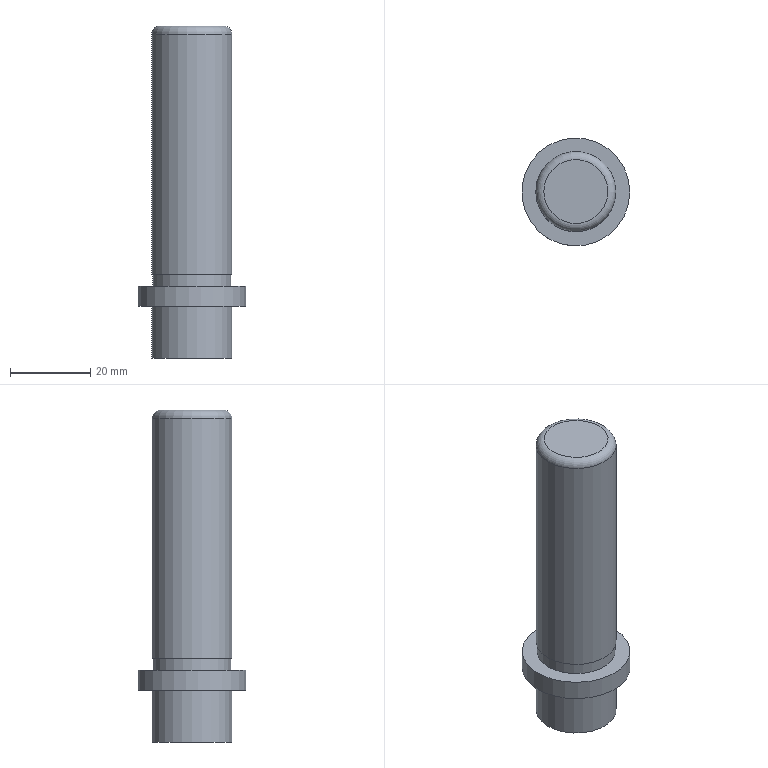Part | NX | features 1 2 | 1 solid | 14 faces | box 27 x 27 x 83 mm | volume 26117 mm3 | cylinder 6 | plane 5 | cone 2 | torus 1 | commonest cylinder face diameters 20 x2 6.8 x1 8 x1 19.5 x1 27 x1
STEP:
#1=CARTESIAN_POINT('',(336.,108.,27.));
#2=VERTEX_POINT('',#1);
#3=CARTESIAN_POINT('',(326.,108.,27.));
#4=DIRECTION('',(0.,0.,1.));
#5=DIRECTION('',(1.,0.,0.));
#6=AXIS2_PLACEMENT_3D('',#3,#4,#5);
#7=CIRCLE('',#6,10.);
#8=EDGE_CURVE('',#2,#2,#7,.T.);
#9=ORIENTED_EDGE('',*,*,#8,.T.);
#10=EDGE_LOOP('',(#9));
#11=FACE_BOUND('',#10,.T.);
#12=CARTESIAN_POINT('',(336.,108.,40.));
#13=VERTEX_POINT('',#12);
#14=CARTESIAN_POINT('',(326.,108.,40.));
#15=DIRECTION('',(0.,0.,1.));
#16=DIRECTION('',(1.,0.,0.));
#17=AXIS2_PLACEMENT_3D('',#14,#15,#16);
#18=CIRCLE('',#17,10.);
#19=EDGE_CURVE('',#13,#13,#18,.T.);
#20=ORIENTED_EDGE('',*,*,#19,.F.);
#21=EDGE_LOOP('',(#20));
#22=FACE_BOUND('',#21,.T.);
#23=CARTESIAN_POINT('',(326.,108.,67.));
#24=DIRECTION('',(0.,0.,1.));
#25=DIRECTION('',(-1.,0.,0.));
#26=AXIS2_PLACEMENT_3D('',#23,#24,#25);
#27=CYLINDRICAL_SURFACE('',#26,10.);
#28=ADVANCED_FACE('',(#11,#22),#27,.T.);
#29=CARTESIAN_POINT('',(339.5,108.,40.));
#30=VERTEX_POINT('',#29);
#31=CARTESIAN_POINT('',(326.,108.,40.));
#32=DIRECTION('',(0.,0.,1.));
#33=DIRECTION('',(1.,0.,0.));
#34=AXIS2_PLACEMENT_3D('',#31,#32,#33);
#35=CIRCLE('',#34,13.5);
#36=EDGE_CURVE('',#30,#30,#35,.T.);
#37=ORIENTED_EDGE('',*,*,#36,.T.);
#38=EDGE_LOOP('',(#37));
#39=FACE_BOUND('',#38,.T.);
#40=CARTESIAN_POINT('',(339.5,108.,45.));
#41=VERTEX_POINT('',#40);
#42=CARTESIAN_POINT('',(326.,108.,45.));
#43=DIRECTION('',(0.,0.,-1.));
#44=DIRECTION('',(1.,0.,0.));
#45=AXIS2_PLACEMENT_3D('',#42,#43,#44);
#46=CIRCLE('',#45,13.5);
#47=EDGE_CURVE('',#41,#41,#46,.T.);
#48=ORIENTED_EDGE('',*,*,#47,.T.);
#49=EDGE_LOOP('',(#48));
#50=FACE_BOUND('',#49,.T.);
#51=CARTESIAN_POINT('',(326.,108.,42.5));
#52=DIRECTION('',(0.,0.,1.));
#53=DIRECTION('',(-1.,0.,0.));
#54=AXIS2_PLACEMENT_3D('',#51,#52,#53);
#55=CYLINDRICAL_SURFACE('',#54,13.5);
#56=ADVANCED_FACE('',(#39,#50),#55,.T.);
#57=CARTESIAN_POINT('',(335.75,108.,45.));
#58=VERTEX_POINT('',#57);
#59=CARTESIAN_POINT('',(326.,108.,45.));
#60=DIRECTION('',(0.,0.,-1.));
#61=DIRECTION('',(1.,0.,0.));
#62=AXIS2_PLACEMENT_3D('',#59,#60,#61);
#63=CIRCLE('',#62,9.75);
#64=EDGE_CURVE('',#58,#58,#63,.T.);
#65=ORIENTED_EDGE('',*,*,#64,.F.);
#66=EDGE_LOOP('',(#65));
#67=FACE_BOUND('',#66,.T.);
#68=CARTESIAN_POINT('',(335.75,108.,48.));
#69=VERTEX_POINT('',#68);
#70=CARTESIAN_POINT('',(326.,108.,48.));
#71=DIRECTION('',(0.,0.,1.));
#72=DIRECTION('',(1.,0.,0.));
#73=AXIS2_PLACEMENT_3D('',#70,#71,#72);
#74=CIRCLE('',#73,9.75);
#75=EDGE_CURVE('',#69,#69,#74,.T.);
#76=ORIENTED_EDGE('',*,*,#75,.F.);
#77=EDGE_LOOP('',(#76));
#78=FACE_BOUND('',#77,.T.);
#79=CARTESIAN_POINT('',(326.,108.,46.5));
#80=DIRECTION('',(0.,0.,1.));
#81=DIRECTION('',(-1.,0.,0.));
#82=AXIS2_PLACEMENT_3D('',#79,#80,#81);
#83=CYLINDRICAL_SURFACE('',#82,9.75);
#84=ADVANCED_FACE('',(#67,#78),#83,.T.);
#85=CARTESIAN_POINT('',(330.,108.,47.));
#86=VERTEX_POINT('',#85);
#87=CARTESIAN_POINT('',(326.,108.,47.));
#88=DIRECTION('',(0.,0.,-1.));
#89=DIRECTION('',(1.,0.,0.));
#90=AXIS2_PLACEMENT_3D('',#87,#88,#89);
#91=CIRCLE('',#90,4.);
#92=EDGE_CURVE('',#86,#86,#91,.T.);
#93=ORIENTED_EDGE('',*,*,#92,.F.);
#94=EDGE_LOOP('',(#93));
#95=FACE_BOUND('',#94,.T.);
#96=CARTESIAN_POINT('',(330.,108.,27.));
#97=VERTEX_POINT('',#96);
#98=CARTESIAN_POINT('',(326.,108.,27.));
#99=DIRECTION('',(0.,0.,-1.));
#100=DIRECTION('',(1.,0.,0.));
#101=AXIS2_PLACEMENT_3D('',#98,#99,#100);
#102=CIRCLE('',#101,4.);
#103=EDGE_CURVE('',#97,#97,#102,.T.);
#104=ORIENTED_EDGE('',*,*,#103,.T.);
#105=EDGE_LOOP('',(#104));
#106=FACE_BOUND('',#105,.T.);
#107=CARTESIAN_POINT('',(326.,108.,37.));
#108=DIRECTION('',(0.,0.,1.));
#109=DIRECTION('',(-1.,0.,0.));
#110=AXIS2_PLACEMENT_3D('',#107,#108,#109);
#111=CYLINDRICAL_SURFACE('',#110,4.);
#112=ADVANCED_FACE('',(#95,#106),#111,.F.);
#113=CARTESIAN_POINT('',(329.4,108.,47.5));
#114=VERTEX_POINT('',#113);
#115=CARTESIAN_POINT('',(326.,108.,47.5));
#116=DIRECTION('',(0.,0.,-1.));
#117=DIRECTION('',(1.,0.,0.));
#118=AXIS2_PLACEMENT_3D('',#115,#116,#117);
#119=CIRCLE('',#118,3.4);
#120=EDGE_CURVE('',#114,#114,#119,.T.);
#121=ORIENTED_EDGE('',*,*,#120,.F.);
#122=EDGE_LOOP('',(#121));
#123=FACE_BOUND('',#122,.T.);
#124=ORIENTED_EDGE('',*,*,#92,.T.);
#125=EDGE_LOOP('',(#124));
#126=FACE_BOUND('',#125,.T.);
#127=CARTESIAN_POINT('',(326.,108.,47.25));
#128=DIRECTION('',(0.,0.,-1.));
#129=DIRECTION('',(-1.,0.,0.));
#130=AXIS2_PLACEMENT_3D('',#127,#128,#129);
#131=CONICAL_SURFACE('',#130,3.7,0.8761);
#132=ADVANCED_FACE('',(#123,#126),#131,.F.);
#133=CARTESIAN_POINT('',(329.4,108.,49.));
#134=VERTEX_POINT('',#133);
#135=CARTESIAN_POINT('',(326.,108.,49.));
#136=DIRECTION('',(0.,0.,-1.));
#137=DIRECTION('',(1.,0.,0.));
#138=AXIS2_PLACEMENT_3D('',#135,#136,#137);
#139=CIRCLE('',#138,3.4);
#140=EDGE_CURVE('',#134,#134,#139,.T.);
#141=ORIENTED_EDGE('',*,*,#140,.F.);
#142=EDGE_LOOP('',(#141));
#143=FACE_BOUND('',#142,.T.);
#144=ORIENTED_EDGE('',*,*,#120,.T.);
#145=EDGE_LOOP('',(#144));
#146=FACE_BOUND('',#145,.T.);
#147=CARTESIAN_POINT('',(326.,108.,48.25));
#148=DIRECTION('',(0.,0.,1.));
#149=DIRECTION('',(-1.,0.,0.));
#150=AXIS2_PLACEMENT_3D('',#147,#148,#149);
#151=CYLINDRICAL_SURFACE('',#150,3.4);
#152=ADVANCED_FACE('',(#143,#146),#151,.F.);
#153=ORIENTED_EDGE('',*,*,#140,.T.);
#154=EDGE_LOOP('',(#153));
#155=FACE_BOUND('',#154,.T.);
#156=CARTESIAN_POINT('',(326.,108.,54.889));
#157=VERTEX_POINT('',#156);
#158=VERTEX_LOOP('',#157);
#159=FACE_BOUND('',#158,.T.);
#160=CARTESIAN_POINT('',(326.,108.,51.944));
#161=DIRECTION('',(0.,0.,-1.));
#162=DIRECTION('',(-1.,0.,0.));
#163=AXIS2_PLACEMENT_3D('',#160,#161,#162);
#164=CONICAL_SURFACE('',#163,1.7,0.5236);
#165=ADVANCED_FACE('',(#155,#159),#164,.F.);
#166=CARTESIAN_POINT('',(336.,108.,48.));
#167=VERTEX_POINT('',#166);
#168=CARTESIAN_POINT('',(326.,108.,48.));
#169=DIRECTION('',(0.,0.,-1.));
#170=DIRECTION('',(1.,0.,0.));
#171=AXIS2_PLACEMENT_3D('',#168,#169,#170);
#172=CIRCLE('',#171,10.);
#173=EDGE_CURVE('',#167,#167,#172,.T.);
#174=ORIENTED_EDGE('',*,*,#173,.F.);
#175=EDGE_LOOP('',(#174));
#176=FACE_BOUND('',#175,.T.);
#177=CARTESIAN_POINT('',(316.,108.,108.));
#178=VERTEX_POINT('',#177);
#179=CARTESIAN_POINT('',(326.,108.,108.));
#180=DIRECTION('',(0.,0.,1.));
#181=DIRECTION('',(-1.,0.,0.));
#182=AXIS2_PLACEMENT_3D('',#179,#180,#181);
#183=CIRCLE('',#182,10.);
#184=EDGE_CURVE('',#178,#178,#183,.F.);
#185=ORIENTED_EDGE('',*,*,#184,.T.);
#186=EDGE_LOOP('',(#185));
#187=FACE_BOUND('',#186,.T.);
#188=CARTESIAN_POINT('',(326.,108.,67.));
#189=DIRECTION('',(0.,0.,1.));
#190=DIRECTION('',(-1.,0.,0.));
#191=AXIS2_PLACEMENT_3D('',#188,#189,#190);
#192=CYLINDRICAL_SURFACE('',#191,10.);
#193=ADVANCED_FACE('',(#176,#187),#192,.T.);
#194=ORIENTED_EDGE('',*,*,#184,.F.);
#195=EDGE_LOOP('',(#194));
#196=FACE_BOUND('',#195,.T.);
#197=CARTESIAN_POINT('',(318.,108.,110.));
#198=VERTEX_POINT('',#197);
#199=CARTESIAN_POINT('',(326.,108.,110.));
#200=DIRECTION('',(0.,0.,1.));
#201=DIRECTION('',(-1.,0.,0.));
#202=AXIS2_PLACEMENT_3D('',#199,#200,#201);
#203=CIRCLE('',#202,8.);
#204=EDGE_CURVE('',#198,#198,#203,.T.);
#205=ORIENTED_EDGE('',*,*,#204,.F.);
#206=EDGE_LOOP('',(#205));
#207=FACE_BOUND('',#206,.T.);
#208=CARTESIAN_POINT('',(326.,108.,108.));
#209=DIRECTION('',(0.,0.,-1.));
#210=DIRECTION('',(-1.,0.,0.));
#211=AXIS2_PLACEMENT_3D('',#208,#209,#210);
#212=TOROIDAL_SURFACE('',#211,8.,2.);
#213=ADVANCED_FACE('',(#196,#207),#212,.T.);
#214=ORIENTED_EDGE('',*,*,#204,.T.);
#215=EDGE_LOOP('',(#214));
#216=FACE_BOUND('',#215,.T.);
#217=CARTESIAN_POINT('',(326.,108.,110.));
#218=DIRECTION('',(0.,0.,-1.));
#219=DIRECTION('',(1.,0.,0.));
#220=AXIS2_PLACEMENT_3D('',#217,#218,#219);
#221=PLANE('',#220);
#222=ADVANCED_FACE('',(#216),#221,.F.);
#223=ORIENTED_EDGE('',*,*,#75,.T.);
#224=EDGE_LOOP('',(#223));
#225=FACE_BOUND('',#224,.T.);
#226=ORIENTED_EDGE('',*,*,#173,.T.);
#227=EDGE_LOOP('',(#226));
#228=FACE_BOUND('',#227,.T.);
#229=CARTESIAN_POINT('',(326.,108.,48.));
#230=DIRECTION('',(0.,0.,1.));
#231=DIRECTION('',(-1.,0.,0.));
#232=AXIS2_PLACEMENT_3D('',#229,#230,#231);
#233=PLANE('',#232);
#234=ADVANCED_FACE('',(#225,#228),#233,.F.);
#235=ORIENTED_EDGE('',*,*,#36,.F.);
#236=EDGE_LOOP('',(#235));
#237=FACE_BOUND('',#236,.T.);
#238=ORIENTED_EDGE('',*,*,#19,.T.);
#239=EDGE_LOOP('',(#238));
#240=FACE_BOUND('',#239,.T.);
#241=CARTESIAN_POINT('',(326.,108.,40.));
#242=DIRECTION('',(0.,0.,-1.));
#243=DIRECTION('',(1.,0.,0.));
#244=AXIS2_PLACEMENT_3D('',#241,#242,#243);
#245=PLANE('',#244);
#246=ADVANCED_FACE('',(#237,#240),#245,.T.);
#247=ORIENTED_EDGE('',*,*,#64,.T.);
#248=EDGE_LOOP('',(#247));
#249=FACE_BOUND('',#248,.T.);
#250=ORIENTED_EDGE('',*,*,#47,.F.);
#251=EDGE_LOOP('',(#250));
#252=FACE_BOUND('',#251,.T.);
#253=CARTESIAN_POINT('',(326.,108.,45.));
#254=DIRECTION('',(0.,0.,1.));
#255=DIRECTION('',(-1.,0.,0.));
#256=AXIS2_PLACEMENT_3D('',#253,#254,#255);
#257=PLANE('',#256);
#258=ADVANCED_FACE('',(#249,#252),#257,.T.);
#259=ORIENTED_EDGE('',*,*,#103,.F.);
#260=EDGE_LOOP('',(#259));
#261=FACE_BOUND('',#260,.T.);
#262=ORIENTED_EDGE('',*,*,#8,.F.);
#263=EDGE_LOOP('',(#262));
#264=FACE_BOUND('',#263,.T.);
#265=CARTESIAN_POINT('',(326.,108.,27.));
#266=DIRECTION('',(0.,0.,-1.));
#267=DIRECTION('',(1.,0.,0.));
#268=AXIS2_PLACEMENT_3D('',#265,#266,#267);
#269=PLANE('',#268);
#270=ADVANCED_FACE('',(#261,#264),#269,.T.);
#271=CLOSED_SHELL('',(#28,#56,#84,#112,#132,#152,#165,#193,#213,#222,#234,#246,#258,#270));
#272=MANIFOLD_SOLID_BREP('',#271);
#273=(LENGTH_UNIT()NAMED_UNIT(*)SI_UNIT(.MILLI.,.METRE.));
#274=UNCERTAINTY_MEASURE_WITH_UNIT(LENGTH_MEASURE(0.00001),#273,'','');
#275=(NAMED_UNIT(*)PLANE_ANGLE_UNIT()SI_UNIT($,.RADIAN.));
#276=(NAMED_UNIT(*)SI_UNIT($,.STERADIAN.)SOLID_ANGLE_UNIT());
#277=(GEOMETRIC_REPRESENTATION_CONTEXT(3)GLOBAL_UNCERTAINTY_ASSIGNED_CONTEXT((#274))GLOBAL_UNIT_ASSIGNED_CONTEXT((#273,#275,#276))REPRESENTATION_CONTEXT('',''));
#278=ADVANCED_BREP_SHAPE_REPRESENTATION('',(#272),#277);